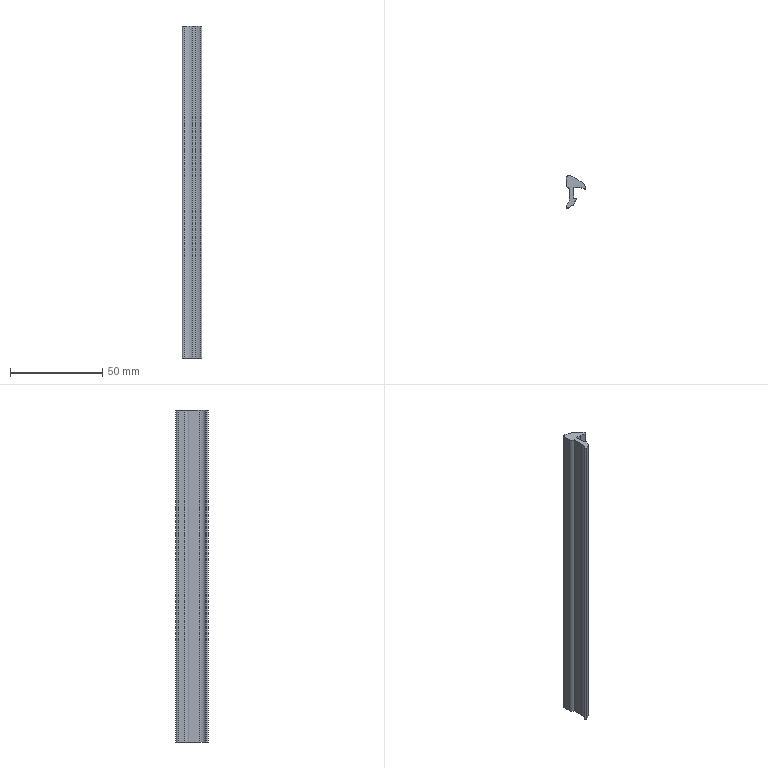Part | SolidWorks | features BaseBody 1, MoveFace 1 | 1 solid | 20 faces | box 10.8 x 17.5 x 180 mm | volume 14184 mm3 | cylinder 11 | plane 9 | commonest cylinder face diameters 1.6 x2 14 x2 0.4 x1 0.6 x1 0.8 x1 2.6 x1
STEP:
#1=CARTESIAN_POINT('',(-3.236,-11.055,80.));
#2=VERTEX_POINT('',#1);
#3=CARTESIAN_POINT('',(-4.3,-10.3,80.));
#4=VERTEX_POINT('',#3);
#5=CARTESIAN_POINT('',(-3.5,-10.3,80.));
#6=DIRECTION('',(0.,0.,-1.));
#7=DIRECTION('',(1.,0.,0.));
#8=AXIS2_PLACEMENT_3D('',#5,#6,#7);
#9=CIRCLE('',#8,0.8);
#10=EDGE_CURVE('',#2,#4,#9,.T.);
#11=ORIENTED_EDGE('',*,*,#10,.T.);
#12=CARTESIAN_POINT('',(-4.3,-10.3,-100.));
#13=VERTEX_POINT('',#12);
#14=CARTESIAN_POINT('',(-4.3,-10.3,-100.));
#15=DIRECTION('',(0.,0.,-1.));
#16=VECTOR('',#15,1000.);
#17=LINE('',#14,#16);
#18=EDGE_CURVE('',#4,#13,#17,.T.);
#19=ORIENTED_EDGE('',*,*,#18,.T.);
#20=CARTESIAN_POINT('',(-3.236,-11.055,-100.));
#21=VERTEX_POINT('',#20);
#22=CARTESIAN_POINT('',(-3.5,-10.3,-100.));
#23=DIRECTION('',(0.,0.,1.));
#24=DIRECTION('',(-1.,0.,0.));
#25=AXIS2_PLACEMENT_3D('',#22,#23,#24);
#26=CIRCLE('',#25,0.8);
#27=EDGE_CURVE('',#13,#21,#26,.T.);
#28=ORIENTED_EDGE('',*,*,#27,.T.);
#29=CARTESIAN_POINT('',(-3.236,-11.055,-100.));
#30=DIRECTION('',(0.,0.,-1.));
#31=VECTOR('',#30,1000.);
#32=LINE('',#29,#31);
#33=EDGE_CURVE('',#2,#21,#32,.T.);
#34=ORIENTED_EDGE('',*,*,#33,.F.);
#35=EDGE_LOOP('',(#11,#19,#28,#34));
#36=FACE_OUTER_BOUND('',#35,.T.);
#37=CARTESIAN_POINT('',(-3.5,-10.3,-100.));
#38=DIRECTION('',(0.,0.,-1.));
#39=DIRECTION('',(-1.,0.,0.));
#40=AXIS2_PLACEMENT_3D('',#37,#38,#39);
#41=CYLINDRICAL_SURFACE('',#40,0.8);
#42=ADVANCED_FACE('',(#36),#41,.T.);
#43=CARTESIAN_POINT('',(1.184,-6.397,-100.));
#44=VERTEX_POINT('',#43);
#45=CARTESIAN_POINT('',(-5.702,-4.29,-100.));
#46=DIRECTION('',(0.,0.,1.));
#47=DIRECTION('',(-1.,0.,0.));
#48=AXIS2_PLACEMENT_3D('',#45,#46,#47);
#49=CIRCLE('',#48,7.201);
#50=EDGE_CURVE('',#21,#44,#49,.T.);
#51=ORIENTED_EDGE('',*,*,#50,.T.);
#52=CARTESIAN_POINT('',(1.184,-6.397,80.));
#53=VERTEX_POINT('',#52);
#54=CARTESIAN_POINT('',(1.184,-6.397,-100.));
#55=DIRECTION('',(0.,0.,1.));
#56=VECTOR('',#55,1000.);
#57=LINE('',#54,#56);
#58=EDGE_CURVE('',#44,#53,#57,.T.);
#59=ORIENTED_EDGE('',*,*,#58,.T.);
#60=CARTESIAN_POINT('',(-5.702,-4.29,80.));
#61=DIRECTION('',(0.,0.,-1.));
#62=DIRECTION('',(1.,0.,0.));
#63=AXIS2_PLACEMENT_3D('',#60,#61,#62);
#64=CIRCLE('',#63,7.201);
#65=EDGE_CURVE('',#53,#2,#64,.T.);
#66=ORIENTED_EDGE('',*,*,#65,.T.);
#67=ORIENTED_EDGE('',*,*,#33,.T.);
#68=EDGE_LOOP('',(#51,#59,#66,#67));
#69=FACE_OUTER_BOUND('',#68,.T.);
#70=CARTESIAN_POINT('',(-5.702,-4.29,-100.));
#71=DIRECTION('',(0.,0.,-1.));
#72=DIRECTION('',(-1.,0.,0.));
#73=AXIS2_PLACEMENT_3D('',#70,#71,#72);
#74=CYLINDRICAL_SURFACE('',#73,7.201);
#75=ADVANCED_FACE('',(#69),#74,.T.);
#76=CARTESIAN_POINT('',(0.9,-6.,-100.));
#77=VERTEX_POINT('',#76);
#78=CARTESIAN_POINT('',(0.9,-6.3,-100.));
#79=DIRECTION('',(0.,0.,1.));
#80=DIRECTION('',(-1.,0.,0.));
#81=AXIS2_PLACEMENT_3D('',#78,#79,#80);
#82=CIRCLE('',#81,0.3);
#83=EDGE_CURVE('',#44,#77,#82,.T.);
#84=ORIENTED_EDGE('',*,*,#83,.T.);
#85=CARTESIAN_POINT('',(0.9,-6.,80.));
#86=VERTEX_POINT('',#85);
#87=CARTESIAN_POINT('',(0.9,-6.,-100.));
#88=DIRECTION('',(0.,0.,1.));
#89=VECTOR('',#88,1000.);
#90=LINE('',#87,#89);
#91=EDGE_CURVE('',#77,#86,#90,.T.);
#92=ORIENTED_EDGE('',*,*,#91,.T.);
#93=CARTESIAN_POINT('',(0.9,-6.3,80.));
#94=DIRECTION('',(0.,0.,-1.));
#95=DIRECTION('',(1.,0.,0.));
#96=AXIS2_PLACEMENT_3D('',#93,#94,#95);
#97=CIRCLE('',#96,0.3);
#98=EDGE_CURVE('',#86,#53,#97,.T.);
#99=ORIENTED_EDGE('',*,*,#98,.T.);
#100=ORIENTED_EDGE('',*,*,#58,.F.);
#101=EDGE_LOOP('',(#84,#92,#99,#100));
#102=FACE_OUTER_BOUND('',#101,.T.);
#103=CARTESIAN_POINT('',(0.9,-6.3,-100.));
#104=DIRECTION('',(0.,0.,-1.));
#105=DIRECTION('',(-1.,0.,0.));
#106=AXIS2_PLACEMENT_3D('',#103,#104,#105);
#107=CYLINDRICAL_SURFACE('',#106,0.3);
#108=ADVANCED_FACE('',(#102),#107,.T.);
#109=CARTESIAN_POINT('',(-2.5,-0.5,-100.));
#110=VERTEX_POINT('',#109);
#111=CARTESIAN_POINT('',(-2.5,-6.153,-100.));
#112=VERTEX_POINT('',#111);
#113=CARTESIAN_POINT('',(-2.5,-6.397,-100.));
#114=DIRECTION('',(0.,-1.,0.));
#115=VECTOR('',#114,1000.);
#116=LINE('',#113,#115);
#117=EDGE_CURVE('',#110,#112,#116,.T.);
#118=ORIENTED_EDGE('',*,*,#117,.F.);
#119=CARTESIAN_POINT('',(-4.2,1.695,-100.));
#120=VERTEX_POINT('',#119);
#121=CARTESIAN_POINT('',(-1.701,1.875,-100.));
#122=DIRECTION('',(0.,0.,1.));
#123=DIRECTION('',(-1.,0.,0.));
#124=AXIS2_PLACEMENT_3D('',#121,#122,#123);
#125=CIRCLE('',#124,2.506);
#126=EDGE_CURVE('',#120,#110,#125,.T.);
#127=ORIENTED_EDGE('',*,*,#126,.F.);
#128=CARTESIAN_POINT('',(-4.2,5.1,-100.));
#129=VERTEX_POINT('',#128);
#130=CARTESIAN_POINT('',(-4.2,-6.397,-100.));
#131=DIRECTION('',(0.,-1.,0.));
#132=VECTOR('',#131,1000.);
#133=LINE('',#130,#132);
#134=EDGE_CURVE('',#129,#120,#133,.T.);
#135=ORIENTED_EDGE('',*,*,#134,.F.);
#136=CARTESIAN_POINT('',(-2.892,6.4,-100.));
#137=VERTEX_POINT('',#136);
#138=CARTESIAN_POINT('',(-2.9,5.1,-100.));
#139=DIRECTION('',(0.,0.,1.));
#140=DIRECTION('',(-1.,0.,0.));
#141=AXIS2_PLACEMENT_3D('',#138,#139,#140);
#142=CIRCLE('',#141,1.3);
#143=EDGE_CURVE('',#137,#129,#142,.T.);
#144=ORIENTED_EDGE('',*,*,#143,.F.);
#145=CARTESIAN_POINT('',(0.5,5.5,-100.));
#146=VERTEX_POINT('',#145);
#147=CARTESIAN_POINT('',(-2.934,-0.5999,-100.));
#148=DIRECTION('',(0.,0.,1.));
#149=DIRECTION('',(-1.,0.,0.));
#150=AXIS2_PLACEMENT_3D('',#147,#148,#149);
#151=CIRCLE('',#150,7.);
#152=EDGE_CURVE('',#146,#137,#151,.T.);
#153=ORIENTED_EDGE('',*,*,#152,.F.);
#154=CARTESIAN_POINT('',(5.5,1.7,-100.));
#155=VERTEX_POINT('',#154);
#156=CARTESIAN_POINT('',(5.5,1.7,-100.));
#157=DIRECTION('',(-0.7962,0.6051,0.));
#158=VECTOR('',#157,1000.);
#159=LINE('',#156,#158);
#160=EDGE_CURVE('',#155,#146,#159,.T.);
#161=ORIENTED_EDGE('',*,*,#160,.F.);
#162=CARTESIAN_POINT('',(6.458,-0.2215,-100.));
#163=VERTEX_POINT('',#162);
#164=CARTESIAN_POINT('',(6.458,-0.2215,-100.));
#165=DIRECTION('',(-0.4462,0.8949,0.));
#166=VECTOR('',#165,1000.);
#167=LINE('',#164,#166);
#168=EDGE_CURVE('',#163,#155,#167,.T.);
#169=ORIENTED_EDGE('',*,*,#168,.F.);
#170=CARTESIAN_POINT('',(5.895,-0.7433,-100.));
#171=VERTEX_POINT('',#170);
#172=CARTESIAN_POINT('',(6.1,-0.4,-100.));
#173=DIRECTION('',(0.,0.,1.));
#174=DIRECTION('',(-1.,0.,0.));
#175=AXIS2_PLACEMENT_3D('',#172,#173,#174);
#176=CIRCLE('',#175,0.4);
#177=EDGE_CURVE('',#171,#163,#176,.T.);
#178=ORIENTED_EDGE('',*,*,#177,.F.);
#179=CARTESIAN_POINT('',(3.,0.,-100.));
#180=VERTEX_POINT('',#179);
#181=CARTESIAN_POINT('',(2.746,-6.995,-100.));
#182=DIRECTION('',(0.,0.,-1.));
#183=DIRECTION('',(-1.,0.,0.));
#184=AXIS2_PLACEMENT_3D('',#181,#182,#183);
#185=CIRCLE('',#184,7.);
#186=EDGE_CURVE('',#180,#171,#185,.T.);
#187=ORIENTED_EDGE('',*,*,#186,.F.);
#188=CARTESIAN_POINT('',(0.,0.,-100.));
#189=VERTEX_POINT('',#188);
#190=CARTESIAN_POINT('',(-6.814,0.,-100.));
#191=DIRECTION('',(1.,0.,0.));
#192=VECTOR('',#191,1000.);
#193=LINE('',#190,#192);
#194=EDGE_CURVE('',#189,#180,#193,.T.);
#195=ORIENTED_EDGE('',*,*,#194,.F.);
#196=CARTESIAN_POINT('',(0.,-5.8,-100.));
#197=VERTEX_POINT('',#196);
#198=CARTESIAN_POINT('',(0.,-6.397,-100.));
#199=DIRECTION('',(0.,1.,0.));
#200=VECTOR('',#199,1000.);
#201=LINE('',#198,#200);
#202=EDGE_CURVE('',#197,#189,#201,.T.);
#203=ORIENTED_EDGE('',*,*,#202,.F.);
#204=CARTESIAN_POINT('',(0.2,-6.,-100.));
#205=VERTEX_POINT('',#204);
#206=CARTESIAN_POINT('',(0.2,-5.8,-100.));
#207=DIRECTION('',(0.,0.,1.));
#208=DIRECTION('',(-1.,0.,0.));
#209=AXIS2_PLACEMENT_3D('',#206,#207,#208);
#210=CIRCLE('',#209,0.2);
#211=EDGE_CURVE('',#197,#205,#210,.T.);
#212=ORIENTED_EDGE('',*,*,#211,.T.);
#213=CARTESIAN_POINT('',(-6.814,-6.,-100.));
#214=DIRECTION('',(-1.,0.,0.));
#215=VECTOR('',#214,1000.);
#216=LINE('',#213,#215);
#217=EDGE_CURVE('',#77,#205,#216,.T.);
#218=ORIENTED_EDGE('',*,*,#217,.F.);
#219=ORIENTED_EDGE('',*,*,#83,.F.);
#220=ORIENTED_EDGE('',*,*,#50,.F.);
#221=ORIENTED_EDGE('',*,*,#27,.F.);
#222=CARTESIAN_POINT('',(-3.998,-9.674,-100.));
#223=VERTEX_POINT('',#222);
#224=CARTESIAN_POINT('',(-3.5,-10.3,-100.));
#225=DIRECTION('',(0.,0.,1.));
#226=DIRECTION('',(-1.,0.,0.));
#227=AXIS2_PLACEMENT_3D('',#224,#225,#226);
#228=CIRCLE('',#227,0.8);
#229=EDGE_CURVE('',#223,#13,#228,.T.);
#230=ORIENTED_EDGE('',*,*,#229,.F.);
#231=CARTESIAN_POINT('',(-6.814,-6.397,-100.));
#232=DIRECTION('',(0.,0.,-1.));
#233=DIRECTION('',(-1.,0.,0.));
#234=AXIS2_PLACEMENT_3D('',#231,#232,#233);
#235=CIRCLE('',#234,4.321);
#236=EDGE_CURVE('',#112,#223,#235,.T.);
#237=ORIENTED_EDGE('',*,*,#236,.F.);
#238=EDGE_LOOP('',(#118,#127,#135,#144,#153,#161,#169,#178,#187,#195,#203,#212,#218,#219,#220,#221,#230,#237));
#239=FACE_OUTER_BOUND('',#238,.T.);
#240=CARTESIAN_POINT('',(-6.814,-6.397,-100.));
#241=DIRECTION('',(0.,0.,1.));
#242=DIRECTION('',(1.,0.,0.));
#243=AXIS2_PLACEMENT_3D('',#240,#241,#242);
#244=PLANE('',#243);
#245=ADVANCED_FACE('',(#239),#244,.F.);
#246=ORIENTED_EDGE('',*,*,#18,.F.);
#247=CARTESIAN_POINT('',(-3.998,-9.674,80.));
#248=VERTEX_POINT('',#247);
#249=CARTESIAN_POINT('',(-3.5,-10.3,80.));
#250=DIRECTION('',(0.,0.,-1.));
#251=DIRECTION('',(1.,0.,0.));
#252=AXIS2_PLACEMENT_3D('',#249,#250,#251);
#253=CIRCLE('',#252,0.8);
#254=EDGE_CURVE('',#4,#248,#253,.T.);
#255=ORIENTED_EDGE('',*,*,#254,.T.);
#256=CARTESIAN_POINT('',(-3.998,-9.674,-100.));
#257=DIRECTION('',(0.,0.,-1.));
#258=VECTOR('',#257,1000.);
#259=LINE('',#256,#258);
#260=EDGE_CURVE('',#248,#223,#259,.T.);
#261=ORIENTED_EDGE('',*,*,#260,.T.);
#262=ORIENTED_EDGE('',*,*,#229,.T.);
#263=EDGE_LOOP('',(#246,#255,#261,#262));
#264=FACE_OUTER_BOUND('',#263,.T.);
#265=CARTESIAN_POINT('',(-3.5,-10.3,-100.));
#266=DIRECTION('',(0.,0.,-1.));
#267=DIRECTION('',(-1.,0.,0.));
#268=AXIS2_PLACEMENT_3D('',#265,#266,#267);
#269=CYLINDRICAL_SURFACE('',#268,0.8);
#270=ADVANCED_FACE('',(#264),#269,.T.);
#271=CARTESIAN_POINT('',(-4.2,1.695,80.));
#272=VERTEX_POINT('',#271);
#273=CARTESIAN_POINT('',(-2.5,-0.5,80.));
#274=VERTEX_POINT('',#273);
#275=CARTESIAN_POINT('',(-1.701,1.875,80.));
#276=DIRECTION('',(0.,0.,1.));
#277=DIRECTION('',(1.,0.,0.));
#278=AXIS2_PLACEMENT_3D('',#275,#276,#277);
#279=CIRCLE('',#278,2.506);
#280=EDGE_CURVE('',#272,#274,#279,.T.);
#281=ORIENTED_EDGE('',*,*,#280,.T.);
#282=CARTESIAN_POINT('',(-2.5,-6.153,80.));
#283=VERTEX_POINT('',#282);
#284=CARTESIAN_POINT('',(-2.5,-6.397,80.));
#285=DIRECTION('',(0.,-1.,0.));
#286=VECTOR('',#285,1000.);
#287=LINE('',#284,#286);
#288=EDGE_CURVE('',#274,#283,#287,.T.);
#289=ORIENTED_EDGE('',*,*,#288,.T.);
#290=CARTESIAN_POINT('',(-6.814,-6.397,80.));
#291=DIRECTION('',(0.,0.,-1.));
#292=DIRECTION('',(1.,0.,0.));
#293=AXIS2_PLACEMENT_3D('',#290,#291,#292);
#294=CIRCLE('',#293,4.321);
#295=EDGE_CURVE('',#283,#248,#294,.T.);
#296=ORIENTED_EDGE('',*,*,#295,.T.);
#297=ORIENTED_EDGE('',*,*,#254,.F.);
#298=ORIENTED_EDGE('',*,*,#10,.F.);
#299=ORIENTED_EDGE('',*,*,#65,.F.);
#300=ORIENTED_EDGE('',*,*,#98,.F.);
#301=CARTESIAN_POINT('',(0.2,-6.,80.));
#302=VERTEX_POINT('',#301);
#303=CARTESIAN_POINT('',(-6.814,-6.,80.));
#304=DIRECTION('',(-1.,0.,0.));
#305=VECTOR('',#304,1000.);
#306=LINE('',#303,#305);
#307=EDGE_CURVE('',#86,#302,#306,.T.);
#308=ORIENTED_EDGE('',*,*,#307,.T.);
#309=CARTESIAN_POINT('',(0.,-5.8,80.));
#310=VERTEX_POINT('',#309);
#311=CARTESIAN_POINT('',(0.2,-5.8,80.));
#312=DIRECTION('',(0.,0.,-1.));
#313=DIRECTION('',(1.,0.,0.));
#314=AXIS2_PLACEMENT_3D('',#311,#312,#313);
#315=CIRCLE('',#314,0.2);
#316=EDGE_CURVE('',#302,#310,#315,.T.);
#317=ORIENTED_EDGE('',*,*,#316,.T.);
#318=CARTESIAN_POINT('',(0.,0.,80.));
#319=VERTEX_POINT('',#318);
#320=CARTESIAN_POINT('',(0.,-6.397,80.));
#321=DIRECTION('',(0.,1.,0.));
#322=VECTOR('',#321,1000.);
#323=LINE('',#320,#322);
#324=EDGE_CURVE('',#310,#319,#323,.T.);
#325=ORIENTED_EDGE('',*,*,#324,.T.);
#326=CARTESIAN_POINT('',(3.,0.,80.));
#327=VERTEX_POINT('',#326);
#328=CARTESIAN_POINT('',(-6.814,0.,80.));
#329=DIRECTION('',(1.,0.,0.));
#330=VECTOR('',#329,1000.);
#331=LINE('',#328,#330);
#332=EDGE_CURVE('',#319,#327,#331,.T.);
#333=ORIENTED_EDGE('',*,*,#332,.T.);
#334=CARTESIAN_POINT('',(5.895,-0.7433,80.));
#335=VERTEX_POINT('',#334);
#336=CARTESIAN_POINT('',(2.746,-6.995,80.));
#337=DIRECTION('',(0.,0.,-1.));
#338=DIRECTION('',(1.,0.,0.));
#339=AXIS2_PLACEMENT_3D('',#336,#337,#338);
#340=CIRCLE('',#339,7.);
#341=EDGE_CURVE('',#327,#335,#340,.T.);
#342=ORIENTED_EDGE('',*,*,#341,.T.);
#343=CARTESIAN_POINT('',(6.458,-0.2215,80.));
#344=VERTEX_POINT('',#343);
#345=CARTESIAN_POINT('',(6.1,-0.4,80.));
#346=DIRECTION('',(0.,0.,-1.));
#347=DIRECTION('',(1.,0.,0.));
#348=AXIS2_PLACEMENT_3D('',#345,#346,#347);
#349=CIRCLE('',#348,0.4);
#350=EDGE_CURVE('',#344,#335,#349,.T.);
#351=ORIENTED_EDGE('',*,*,#350,.F.);
#352=CARTESIAN_POINT('',(5.5,1.7,80.));
#353=VERTEX_POINT('',#352);
#354=CARTESIAN_POINT('',(6.282,0.1323,80.));
#355=DIRECTION('',(-0.4462,0.8949,0.));
#356=VECTOR('',#355,1000.);
#357=LINE('',#354,#356);
#358=EDGE_CURVE('',#344,#353,#357,.T.);
#359=ORIENTED_EDGE('',*,*,#358,.T.);
#360=CARTESIAN_POINT('',(0.5,5.5,80.));
#361=VERTEX_POINT('',#360);
#362=CARTESIAN_POINT('',(1.595,4.668,80.));
#363=DIRECTION('',(-0.7962,0.6051,0.));
#364=VECTOR('',#363,1000.);
#365=LINE('',#362,#364);
#366=EDGE_CURVE('',#353,#361,#365,.T.);
#367=ORIENTED_EDGE('',*,*,#366,.T.);
#368=CARTESIAN_POINT('',(-2.892,6.4,80.));
#369=VERTEX_POINT('',#368);
#370=CARTESIAN_POINT('',(-2.934,-0.5999,80.));
#371=DIRECTION('',(0.,0.,1.));
#372=DIRECTION('',(1.,0.,0.));
#373=AXIS2_PLACEMENT_3D('',#370,#371,#372);
#374=CIRCLE('',#373,7.);
#375=EDGE_CURVE('',#361,#369,#374,.T.);
#376=ORIENTED_EDGE('',*,*,#375,.T.);
#377=CARTESIAN_POINT('',(-4.2,5.1,80.));
#378=VERTEX_POINT('',#377);
#379=CARTESIAN_POINT('',(-2.9,5.1,80.));
#380=DIRECTION('',(0.,0.,1.));
#381=DIRECTION('',(1.,0.,0.));
#382=AXIS2_PLACEMENT_3D('',#379,#380,#381);
#383=CIRCLE('',#382,1.3);
#384=EDGE_CURVE('',#369,#378,#383,.T.);
#385=ORIENTED_EDGE('',*,*,#384,.T.);
#386=CARTESIAN_POINT('',(-4.2,-6.397,80.));
#387=DIRECTION('',(0.,-1.,0.));
#388=VECTOR('',#387,1000.);
#389=LINE('',#386,#388);
#390=EDGE_CURVE('',#378,#272,#389,.T.);
#391=ORIENTED_EDGE('',*,*,#390,.T.);
#392=EDGE_LOOP('',(#281,#289,#296,#297,#298,#299,#300,#308,#317,#325,#333,#342,#351,#359,#367,#376,#385,#391));
#393=FACE_OUTER_BOUND('',#392,.T.);
#394=CARTESIAN_POINT('',(-6.814,-6.397,80.));
#395=DIRECTION('',(0.,0.,1.));
#396=DIRECTION('',(1.,0.,0.));
#397=AXIS2_PLACEMENT_3D('',#394,#395,#396);
#398=PLANE('',#397);
#399=ADVANCED_FACE('',(#393),#398,.T.);
#400=ORIENTED_EDGE('',*,*,#217,.T.);
#401=CARTESIAN_POINT('',(0.2,-6.,-100.));
#402=DIRECTION('',(0.,0.,1.));
#403=VECTOR('',#402,1000.);
#404=LINE('',#401,#403);
#405=EDGE_CURVE('',#205,#302,#404,.T.);
#406=ORIENTED_EDGE('',*,*,#405,.T.);
#407=ORIENTED_EDGE('',*,*,#307,.F.);
#408=ORIENTED_EDGE('',*,*,#91,.F.);
#409=EDGE_LOOP('',(#400,#406,#407,#408));
#410=FACE_OUTER_BOUND('',#409,.T.);
#411=CARTESIAN_POINT('',(0.9,-6.,-100.));
#412=DIRECTION('',(0.,1.,0.));
#413=DIRECTION('',(0.,0.,1.));
#414=AXIS2_PLACEMENT_3D('',#411,#412,#413);
#415=PLANE('',#414);
#416=ADVANCED_FACE('',(#410),#415,.T.);
#417=CARTESIAN_POINT('',(-2.5,-6.153,-100.));
#418=DIRECTION('',(0.,0.,1.));
#419=VECTOR('',#418,1000.);
#420=LINE('',#417,#419);
#421=EDGE_CURVE('',#112,#283,#420,.T.);
#422=ORIENTED_EDGE('',*,*,#421,.F.);
#423=ORIENTED_EDGE('',*,*,#236,.T.);
#424=ORIENTED_EDGE('',*,*,#260,.F.);
#425=ORIENTED_EDGE('',*,*,#295,.F.);
#426=EDGE_LOOP('',(#422,#423,#424,#425));
#427=FACE_OUTER_BOUND('',#426,.T.);
#428=CARTESIAN_POINT('',(-6.814,-6.397,-100.));
#429=DIRECTION('',(0.,0.,-1.));
#430=DIRECTION('',(-1.,0.,0.));
#431=AXIS2_PLACEMENT_3D('',#428,#429,#430);
#432=CYLINDRICAL_SURFACE('',#431,4.321);
#433=ADVANCED_FACE('',(#427),#432,.F.);
#434=ORIENTED_EDGE('',*,*,#117,.T.);
#435=ORIENTED_EDGE('',*,*,#421,.T.);
#436=ORIENTED_EDGE('',*,*,#288,.F.);
#437=CARTESIAN_POINT('',(-2.5,-0.5,-100.));
#438=DIRECTION('',(0.,0.,-1.));
#439=VECTOR('',#438,1000.);
#440=LINE('',#437,#439);
#441=EDGE_CURVE('',#274,#110,#440,.T.);
#442=ORIENTED_EDGE('',*,*,#441,.T.);
#443=EDGE_LOOP('',(#434,#435,#436,#442));
#444=FACE_OUTER_BOUND('',#443,.T.);
#445=CARTESIAN_POINT('',(-2.5,-0.5,-100.));
#446=DIRECTION('',(-1.,0.,0.));
#447=DIRECTION('',(0.,0.,1.));
#448=AXIS2_PLACEMENT_3D('',#445,#446,#447);
#449=PLANE('',#448);
#450=ADVANCED_FACE('',(#444),#449,.T.);
#451=ORIENTED_EDGE('',*,*,#126,.T.);
#452=ORIENTED_EDGE('',*,*,#441,.F.);
#453=ORIENTED_EDGE('',*,*,#280,.F.);
#454=CARTESIAN_POINT('',(-4.2,1.695,-100.));
#455=DIRECTION('',(0.,0.,-1.));
#456=VECTOR('',#455,1000.);
#457=LINE('',#454,#456);
#458=EDGE_CURVE('',#272,#120,#457,.T.);
#459=ORIENTED_EDGE('',*,*,#458,.T.);
#460=EDGE_LOOP('',(#451,#452,#453,#459));
#461=FACE_OUTER_BOUND('',#460,.T.);
#462=CARTESIAN_POINT('',(-1.701,1.875,-100.));
#463=DIRECTION('',(0.,0.,-1.));
#464=DIRECTION('',(-1.,0.,0.));
#465=AXIS2_PLACEMENT_3D('',#462,#463,#464);
#466=CYLINDRICAL_SURFACE('',#465,2.506);
#467=ADVANCED_FACE('',(#461),#466,.T.);
#468=ORIENTED_EDGE('',*,*,#134,.T.);
#469=ORIENTED_EDGE('',*,*,#458,.F.);
#470=ORIENTED_EDGE('',*,*,#390,.F.);
#471=CARTESIAN_POINT('',(-4.2,5.1,-100.));
#472=DIRECTION('',(0.,0.,-1.));
#473=VECTOR('',#472,1000.);
#474=LINE('',#471,#473);
#475=EDGE_CURVE('',#378,#129,#474,.T.);
#476=ORIENTED_EDGE('',*,*,#475,.T.);
#477=EDGE_LOOP('',(#468,#469,#470,#476));
#478=FACE_OUTER_BOUND('',#477,.T.);
#479=CARTESIAN_POINT('',(-4.2,5.1,-100.));
#480=DIRECTION('',(-1.,0.,0.));
#481=DIRECTION('',(0.,0.,1.));
#482=AXIS2_PLACEMENT_3D('',#479,#480,#481);
#483=PLANE('',#482);
#484=ADVANCED_FACE('',(#478),#483,.T.);
#485=ORIENTED_EDGE('',*,*,#143,.T.);
#486=ORIENTED_EDGE('',*,*,#475,.F.);
#487=ORIENTED_EDGE('',*,*,#384,.F.);
#488=CARTESIAN_POINT('',(-2.892,6.4,-100.));
#489=DIRECTION('',(0.,0.,-1.));
#490=VECTOR('',#489,1000.);
#491=LINE('',#488,#490);
#492=EDGE_CURVE('',#369,#137,#491,.T.);
#493=ORIENTED_EDGE('',*,*,#492,.T.);
#494=EDGE_LOOP('',(#485,#486,#487,#493));
#495=FACE_OUTER_BOUND('',#494,.T.);
#496=CARTESIAN_POINT('',(-2.9,5.1,-100.));
#497=DIRECTION('',(0.,0.,-1.));
#498=DIRECTION('',(-1.,0.,0.));
#499=AXIS2_PLACEMENT_3D('',#496,#497,#498);
#500=CYLINDRICAL_SURFACE('',#499,1.3);
#501=ADVANCED_FACE('',(#495),#500,.T.);
#502=ORIENTED_EDGE('',*,*,#152,.T.);
#503=ORIENTED_EDGE('',*,*,#492,.F.);
#504=ORIENTED_EDGE('',*,*,#375,.F.);
#505=CARTESIAN_POINT('',(0.5,5.5,-100.));
#506=DIRECTION('',(0.,0.,-1.));
#507=VECTOR('',#506,1000.);
#508=LINE('',#505,#507);
#509=EDGE_CURVE('',#361,#146,#508,.T.);
#510=ORIENTED_EDGE('',*,*,#509,.T.);
#511=EDGE_LOOP('',(#502,#503,#504,#510));
#512=FACE_OUTER_BOUND('',#511,.T.);
#513=CARTESIAN_POINT('',(-2.934,-0.5999,-100.));
#514=DIRECTION('',(0.,0.,-1.));
#515=DIRECTION('',(-1.,0.,0.));
#516=AXIS2_PLACEMENT_3D('',#513,#514,#515);
#517=CYLINDRICAL_SURFACE('',#516,7.);
#518=ADVANCED_FACE('',(#512),#517,.T.);
#519=ORIENTED_EDGE('',*,*,#160,.T.);
#520=ORIENTED_EDGE('',*,*,#509,.F.);
#521=ORIENTED_EDGE('',*,*,#366,.F.);
#522=CARTESIAN_POINT('',(5.5,1.7,-100.));
#523=DIRECTION('',(0.,0.,-1.));
#524=VECTOR('',#523,1000.);
#525=LINE('',#522,#524);
#526=EDGE_CURVE('',#353,#155,#525,.T.);
#527=ORIENTED_EDGE('',*,*,#526,.T.);
#528=EDGE_LOOP('',(#519,#520,#521,#527));
#529=FACE_OUTER_BOUND('',#528,.T.);
#530=CARTESIAN_POINT('',(5.5,1.7,-100.));
#531=DIRECTION('',(0.6051,0.7962,0.));
#532=DIRECTION('',(-0.7962,0.6051,0.));
#533=AXIS2_PLACEMENT_3D('',#530,#531,#532);
#534=PLANE('',#533);
#535=ADVANCED_FACE('',(#529),#534,.T.);
#536=ORIENTED_EDGE('',*,*,#168,.T.);
#537=ORIENTED_EDGE('',*,*,#526,.F.);
#538=ORIENTED_EDGE('',*,*,#358,.F.);
#539=CARTESIAN_POINT('',(6.458,-0.2215,-100.));
#540=DIRECTION('',(0.,0.,-1.));
#541=VECTOR('',#540,1000.);
#542=LINE('',#539,#541);
#543=EDGE_CURVE('',#344,#163,#542,.T.);
#544=ORIENTED_EDGE('',*,*,#543,.T.);
#545=EDGE_LOOP('',(#536,#537,#538,#544));
#546=FACE_OUTER_BOUND('',#545,.T.);
#547=CARTESIAN_POINT('',(6.458,-0.2215,-100.));
#548=DIRECTION('',(0.8949,0.4462,0.));
#549=DIRECTION('',(-0.4462,0.8949,0.));
#550=AXIS2_PLACEMENT_3D('',#547,#548,#549);
#551=PLANE('',#550);
#552=ADVANCED_FACE('',(#546),#551,.T.);
#553=CARTESIAN_POINT('',(3.,0.,-100.));
#554=DIRECTION('',(0.,0.,1.));
#555=VECTOR('',#554,1000.);
#556=LINE('',#553,#555);
#557=EDGE_CURVE('',#180,#327,#556,.T.);
#558=ORIENTED_EDGE('',*,*,#557,.F.);
#559=ORIENTED_EDGE('',*,*,#186,.T.);
#560=CARTESIAN_POINT('',(5.895,-0.7433,-100.));
#561=DIRECTION('',(0.,0.,-1.));
#562=VECTOR('',#561,1000.);
#563=LINE('',#560,#562);
#564=EDGE_CURVE('',#335,#171,#563,.T.);
#565=ORIENTED_EDGE('',*,*,#564,.F.);
#566=ORIENTED_EDGE('',*,*,#341,.F.);
#567=EDGE_LOOP('',(#558,#559,#565,#566));
#568=FACE_OUTER_BOUND('',#567,.T.);
#569=CARTESIAN_POINT('',(2.746,-6.995,-100.));
#570=DIRECTION('',(0.,0.,-1.));
#571=DIRECTION('',(-1.,0.,0.));
#572=AXIS2_PLACEMENT_3D('',#569,#570,#571);
#573=CYLINDRICAL_SURFACE('',#572,7.);
#574=ADVANCED_FACE('',(#568),#573,.F.);
#575=ORIENTED_EDGE('',*,*,#194,.T.);
#576=ORIENTED_EDGE('',*,*,#557,.T.);
#577=ORIENTED_EDGE('',*,*,#332,.F.);
#578=CARTESIAN_POINT('',(0.,0.,-100.));
#579=DIRECTION('',(0.,0.,-1.));
#580=VECTOR('',#579,1000.);
#581=LINE('',#578,#580);
#582=EDGE_CURVE('',#319,#189,#581,.T.);
#583=ORIENTED_EDGE('',*,*,#582,.T.);
#584=EDGE_LOOP('',(#575,#576,#577,#583));
#585=FACE_OUTER_BOUND('',#584,.T.);
#586=CARTESIAN_POINT('',(0.,0.,-100.));
#587=DIRECTION('',(0.,-1.,0.));
#588=DIRECTION('',(0.,0.,-1.));
#589=AXIS2_PLACEMENT_3D('',#586,#587,#588);
#590=PLANE('',#589);
#591=ADVANCED_FACE('',(#585),#590,.T.);
#592=ORIENTED_EDGE('',*,*,#202,.T.);
#593=ORIENTED_EDGE('',*,*,#582,.F.);
#594=ORIENTED_EDGE('',*,*,#324,.F.);
#595=CARTESIAN_POINT('',(0.,-5.8,-100.));
#596=DIRECTION('',(0.,0.,-1.));
#597=VECTOR('',#596,1000.);
#598=LINE('',#595,#597);
#599=EDGE_CURVE('',#310,#197,#598,.T.);
#600=ORIENTED_EDGE('',*,*,#599,.T.);
#601=EDGE_LOOP('',(#592,#593,#594,#600));
#602=FACE_OUTER_BOUND('',#601,.T.);
#603=CARTESIAN_POINT('',(0.,-5.8,-100.));
#604=DIRECTION('',(1.,0.,0.));
#605=DIRECTION('',(0.,0.,-1.));
#606=AXIS2_PLACEMENT_3D('',#603,#604,#605);
#607=PLANE('',#606);
#608=ADVANCED_FACE('',(#602),#607,.T.);
#609=ORIENTED_EDGE('',*,*,#405,.F.);
#610=ORIENTED_EDGE('',*,*,#211,.F.);
#611=ORIENTED_EDGE('',*,*,#599,.F.);
#612=ORIENTED_EDGE('',*,*,#316,.F.);
#613=EDGE_LOOP('',(#609,#610,#611,#612));
#614=FACE_OUTER_BOUND('',#613,.T.);
#615=CARTESIAN_POINT('',(0.2,-5.8,-100.));
#616=DIRECTION('',(0.,0.,-1.));
#617=DIRECTION('',(-1.,0.,0.));
#618=AXIS2_PLACEMENT_3D('',#615,#616,#617);
#619=CYLINDRICAL_SURFACE('',#618,0.2);
#620=ADVANCED_FACE('',(#614),#619,.F.);
#621=ORIENTED_EDGE('',*,*,#177,.T.);
#622=ORIENTED_EDGE('',*,*,#543,.F.);
#623=ORIENTED_EDGE('',*,*,#350,.T.);
#624=ORIENTED_EDGE('',*,*,#564,.T.);
#625=EDGE_LOOP('',(#621,#622,#623,#624));
#626=FACE_OUTER_BOUND('',#625,.T.);
#627=CARTESIAN_POINT('',(6.1,-0.4,-100.));
#628=DIRECTION('',(0.,0.,-1.));
#629=DIRECTION('',(-1.,0.,0.));
#630=AXIS2_PLACEMENT_3D('',#627,#628,#629);
#631=CYLINDRICAL_SURFACE('',#630,0.4);
#632=ADVANCED_FACE('',(#626),#631,.T.);
#633=CLOSED_SHELL('',(#42,#75,#108,#245,#270,#399,#416,#433,#450,#467,#484,#501,#518,#535,#552,#574,#591,#608,#620,#632));
#634=MANIFOLD_SOLID_BREP('',#633);
#635=CARTESIAN_POINT('',(0.,0.,0.));
#636=DIRECTION('',(0.,0.,1.));
#637=DIRECTION('',(1.,0.,0.));
#638=AXIS2_PLACEMENT_3D('',#635,#636,#637);
#639=(LENGTH_UNIT()NAMED_UNIT(*)SI_UNIT(.MILLI.,.METRE.));
#640=UNCERTAINTY_MEASURE_WITH_UNIT(LENGTH_MEASURE(0.00001),#639,'','');
#641=(NAMED_UNIT(*)PLANE_ANGLE_UNIT()SI_UNIT($,.RADIAN.));
#642=(NAMED_UNIT(*)SI_UNIT($,.STERADIAN.)SOLID_ANGLE_UNIT());
#643=(GEOMETRIC_REPRESENTATION_CONTEXT(3)GLOBAL_UNCERTAINTY_ASSIGNED_CONTEXT((#640))GLOBAL_UNIT_ASSIGNED_CONTEXT((#639,#641,#642))REPRESENTATION_CONTEXT('',''));
#644=ADVANCED_BREP_SHAPE_REPRESENTATION('',(#634,#638),#643);